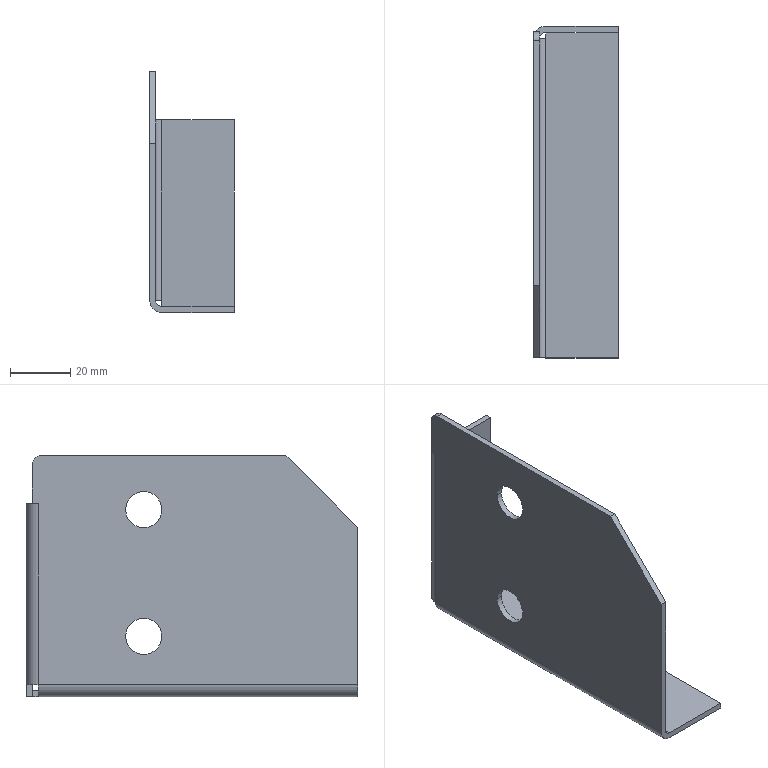Part | NX | features solid 2 | 1 solid | 30 faces | box 28 x 110 x 80 mm | volume 24962 mm3 | plane 21 | cylinder 9 | commonest cylinder face diameters 12 x4 4 x2 8 x2 6 x1
STEP:
#1=CARTESIAN_POINT('',(1138.,-1578.,1213.));
#2=VERTEX_POINT('',#1);
#3=CARTESIAN_POINT('',(1114.,-1578.,1213.));
#4=VERTEX_POINT('',#3);
#5=CARTESIAN_POINT('',(1111.722,-1578.,1213.));
#6=DIRECTION('',(-1.,0.,0.));
#7=VECTOR('',#6,1000.);
#8=LINE('',#5,#7);
#9=EDGE_CURVE('',#2,#4,#8,.T.);
#10=ORIENTED_EDGE('',*,*,#9,.T.);
#11=CARTESIAN_POINT('',(1114.,-1472.,1213.));
#12=VERTEX_POINT('',#11);
#13=CARTESIAN_POINT('',(1114.,-1578.,1213.));
#14=DIRECTION('',(0.,1.,0.));
#15=VECTOR('',#14,1000.);
#16=LINE('',#13,#15);
#17=EDGE_CURVE('',#4,#12,#16,.T.);
#18=ORIENTED_EDGE('',*,*,#17,.T.);
#19=CARTESIAN_POINT('',(1114.,-1470.2,1213.));
#20=VERTEX_POINT('',#19);
#21=CARTESIAN_POINT('',(1114.,-1578.,1213.));
#22=DIRECTION('',(0.,1.,0.));
#23=VECTOR('',#22,1000.);
#24=LINE('',#21,#23);
#25=EDGE_CURVE('',#12,#20,#24,.T.);
#26=ORIENTED_EDGE('',*,*,#25,.T.);
#27=CARTESIAN_POINT('',(1138.,-1470.2,1213.));
#28=VERTEX_POINT('',#27);
#29=CARTESIAN_POINT('',(1111.722,-1470.2,1213.));
#30=DIRECTION('',(1.,0.,0.));
#31=VECTOR('',#30,1000.);
#32=LINE('',#29,#31);
#33=EDGE_CURVE('',#20,#28,#32,.T.);
#34=ORIENTED_EDGE('',*,*,#33,.T.);
#35=CARTESIAN_POINT('',(1138.,-1472.,1213.));
#36=DIRECTION('',(0.,-1.,0.));
#37=VECTOR('',#36,1000.);
#38=LINE('',#35,#37);
#39=EDGE_CURVE('',#28,#2,#38,.T.);
#40=ORIENTED_EDGE('',*,*,#39,.T.);
#41=EDGE_LOOP('',(#10,#18,#26,#34,#40));
#42=FACE_BOUND('',#41,.T.);
#43=CARTESIAN_POINT('',(1110.,-1682.,1213.));
#44=DIRECTION('',(0.,0.,-1.));
#45=DIRECTION('',(0.,-1.,0.));
#46=AXIS2_PLACEMENT_3D('',#43,#44,#45);
#47=PLANE('',#46);
#48=ADVANCED_FACE('',(#42),#47,.T.);
#49=CARTESIAN_POINT('',(1114.,-1578.,1215.));
#50=VERTEX_POINT('',#49);
#51=CARTESIAN_POINT('',(1114.,-1472.,1215.));
#52=VERTEX_POINT('',#51);
#53=CARTESIAN_POINT('',(1114.,-1578.,1215.));
#54=DIRECTION('',(0.,1.,0.));
#55=VECTOR('',#54,1000.);
#56=LINE('',#53,#55);
#57=EDGE_CURVE('',#50,#52,#56,.T.);
#58=ORIENTED_EDGE('',*,*,#57,.F.);
#59=CARTESIAN_POINT('',(1138.,-1578.,1215.));
#60=VERTEX_POINT('',#59);
#61=CARTESIAN_POINT('',(1111.722,-1578.,1215.));
#62=DIRECTION('',(-1.,0.,0.));
#63=VECTOR('',#62,1000.);
#64=LINE('',#61,#63);
#65=EDGE_CURVE('',#60,#50,#64,.T.);
#66=ORIENTED_EDGE('',*,*,#65,.F.);
#67=CARTESIAN_POINT('',(1138.,-1470.2,1215.));
#68=VERTEX_POINT('',#67);
#69=CARTESIAN_POINT('',(1138.,-1472.,1215.));
#70=DIRECTION('',(0.,-1.,0.));
#71=VECTOR('',#70,1000.);
#72=LINE('',#69,#71);
#73=EDGE_CURVE('',#68,#60,#72,.T.);
#74=ORIENTED_EDGE('',*,*,#73,.F.);
#75=CARTESIAN_POINT('',(1114.,-1470.2,1215.));
#76=VERTEX_POINT('',#75);
#77=CARTESIAN_POINT('',(1111.722,-1470.2,1215.));
#78=DIRECTION('',(1.,0.,0.));
#79=VECTOR('',#78,1000.);
#80=LINE('',#77,#79);
#81=EDGE_CURVE('',#76,#68,#80,.T.);
#82=ORIENTED_EDGE('',*,*,#81,.F.);
#83=CARTESIAN_POINT('',(1114.,-1578.,1215.));
#84=DIRECTION('',(0.,1.,0.));
#85=VECTOR('',#84,1000.);
#86=LINE('',#83,#85);
#87=EDGE_CURVE('',#52,#76,#86,.T.);
#88=ORIENTED_EDGE('',*,*,#87,.F.);
#89=EDGE_LOOP('',(#58,#66,#74,#82,#88));
#90=FACE_BOUND('',#89,.T.);
#91=CARTESIAN_POINT('',(1110.,-1682.,1215.));
#92=DIRECTION('',(0.,0.,-1.));
#93=DIRECTION('',(0.,-1.,0.));
#94=AXIS2_PLACEMENT_3D('',#91,#92,#93);
#95=PLANE('',#94);
#96=ADVANCED_FACE('',(#90),#95,.F.);
#97=ORIENTED_EDGE('',*,*,#33,.F.);
#98=CARTESIAN_POINT('',(1114.,-1470.2,1213.));
#99=DIRECTION('',(0.,0.,1.));
#100=VECTOR('',#99,1000.);
#101=LINE('',#98,#100);
#102=EDGE_CURVE('',#20,#76,#101,.T.);
#103=ORIENTED_EDGE('',*,*,#102,.T.);
#104=ORIENTED_EDGE('',*,*,#81,.T.);
#105=CARTESIAN_POINT('',(1138.,-1470.2,1213.));
#106=DIRECTION('',(0.,0.,1.));
#107=VECTOR('',#106,1000.);
#108=LINE('',#105,#107);
#109=EDGE_CURVE('',#28,#68,#108,.T.);
#110=ORIENTED_EDGE('',*,*,#109,.F.);
#111=EDGE_LOOP('',(#97,#103,#104,#110));
#112=FACE_BOUND('',#111,.T.);
#113=CARTESIAN_POINT('',(1111.722,-1470.2,1213.));
#114=DIRECTION('',(0.,-1.,0.));
#115=DIRECTION('',(-1.,0.,0.));
#116=AXIS2_PLACEMENT_3D('',#113,#114,#115);
#117=PLANE('',#116);
#118=ADVANCED_FACE('',(#112),#117,.F.);
#119=ORIENTED_EDGE('',*,*,#73,.T.);
#120=CARTESIAN_POINT('',(1138.,-1578.,1213.));
#121=DIRECTION('',(0.,0.,1.));
#122=VECTOR('',#121,1000.);
#123=LINE('',#120,#122);
#124=EDGE_CURVE('',#2,#60,#123,.T.);
#125=ORIENTED_EDGE('',*,*,#124,.F.);
#126=ORIENTED_EDGE('',*,*,#39,.F.);
#127=ORIENTED_EDGE('',*,*,#109,.T.);
#128=EDGE_LOOP('',(#119,#125,#126,#127));
#129=FACE_BOUND('',#128,.T.);
#130=CARTESIAN_POINT('',(1138.,-1472.,1213.));
#131=DIRECTION('',(-1.,0.,0.));
#132=DIRECTION('',(0.,0.,1.));
#133=AXIS2_PLACEMENT_3D('',#130,#131,#132);
#134=PLANE('',#133);
#135=ADVANCED_FACE('',(#129),#134,.F.);
#136=ORIENTED_EDGE('',*,*,#25,.F.);
#137=CARTESIAN_POINT('',(1114.,-1472.,1213.));
#138=DIRECTION('',(0.,0.,1.));
#139=VECTOR('',#138,1000.);
#140=LINE('',#137,#139);
#141=EDGE_CURVE('',#12,#52,#140,.T.);
#142=ORIENTED_EDGE('',*,*,#141,.T.);
#143=ORIENTED_EDGE('',*,*,#87,.T.);
#144=ORIENTED_EDGE('',*,*,#102,.F.);
#145=EDGE_LOOP('',(#136,#142,#143,#144));
#146=FACE_BOUND('',#145,.T.);
#147=CARTESIAN_POINT('',(1114.,-1682.,0.));
#148=DIRECTION('',(-1.,0.,0.));
#149=DIRECTION('',(0.,1.,0.));
#150=AXIS2_PLACEMENT_3D('',#147,#148,#149);
#151=PLANE('',#150);
#152=ADVANCED_FACE('',(#146),#151,.T.);
#153=CARTESIAN_POINT('',(1110.,-1513.,1275.));
#154=VERTEX_POINT('',#153);
#155=CARTESIAN_POINT('',(1110.,-1501.,1275.));
#156=VERTEX_POINT('',#155);
#157=CARTESIAN_POINT('',(1110.,-1507.,1275.));
#158=DIRECTION('',(1.,0.,0.));
#159=DIRECTION('',(0.,-1.,0.));
#160=AXIS2_PLACEMENT_3D('',#157,#158,#159);
#161=CIRCLE('',#160,6.);
#162=EDGE_CURVE('',#154,#156,#161,.T.);
#163=ORIENTED_EDGE('',*,*,#162,.T.);
#164=CARTESIAN_POINT('',(1110.,-1507.,1275.));
#165=DIRECTION('',(1.,0.,0.));
#166=DIRECTION('',(0.,-1.,0.));
#167=AXIS2_PLACEMENT_3D('',#164,#165,#166);
#168=CIRCLE('',#167,6.);
#169=EDGE_CURVE('',#156,#154,#168,.T.);
#170=ORIENTED_EDGE('',*,*,#169,.T.);
#171=EDGE_LOOP('',(#163,#170));
#172=FACE_BOUND('',#171,.T.);
#173=CARTESIAN_POINT('',(1110.,-1513.,1233.));
#174=VERTEX_POINT('',#173);
#175=CARTESIAN_POINT('',(1110.,-1501.,1233.));
#176=VERTEX_POINT('',#175);
#177=CARTESIAN_POINT('',(1110.,-1507.,1233.));
#178=DIRECTION('',(1.,0.,0.));
#179=DIRECTION('',(0.,-1.,0.));
#180=AXIS2_PLACEMENT_3D('',#177,#178,#179);
#181=CIRCLE('',#180,6.);
#182=EDGE_CURVE('',#174,#176,#181,.T.);
#183=ORIENTED_EDGE('',*,*,#182,.T.);
#184=CARTESIAN_POINT('',(1110.,-1507.,1233.));
#185=DIRECTION('',(1.,0.,0.));
#186=DIRECTION('',(0.,-1.,0.));
#187=AXIS2_PLACEMENT_3D('',#184,#185,#186);
#188=CIRCLE('',#187,6.);
#189=EDGE_CURVE('',#176,#174,#188,.T.);
#190=ORIENTED_EDGE('',*,*,#189,.T.);
#191=EDGE_LOOP('',(#183,#190));
#192=FACE_BOUND('',#191,.T.);
#193=CARTESIAN_POINT('',(1110.,-1472.,1277.));
#194=VERTEX_POINT('',#193);
#195=CARTESIAN_POINT('',(1110.,-1472.,1217.));
#196=VERTEX_POINT('',#195);
#197=CARTESIAN_POINT('',(1110.,-1472.,1277.));
#198=DIRECTION('',(0.,0.,-1.));
#199=VECTOR('',#198,1000.);
#200=LINE('',#197,#199);
#201=EDGE_CURVE('',#194,#196,#200,.T.);
#202=ORIENTED_EDGE('',*,*,#201,.T.);
#203=CARTESIAN_POINT('',(1110.,-1578.,1217.));
#204=VERTEX_POINT('',#203);
#205=CARTESIAN_POINT('',(1110.,-1472.,1217.));
#206=DIRECTION('',(0.,-1.,0.));
#207=VECTOR('',#206,1000.);
#208=LINE('',#205,#207);
#209=EDGE_CURVE('',#196,#204,#208,.T.);
#210=ORIENTED_EDGE('',*,*,#209,.T.);
#211=CARTESIAN_POINT('',(1110.,-1578.,1269.17));
#212=VERTEX_POINT('',#211);
#213=CARTESIAN_POINT('',(1110.,-1578.,1269.17));
#214=DIRECTION('',(0.,0.,-1.));
#215=VECTOR('',#214,1000.);
#216=LINE('',#213,#215);
#217=EDGE_CURVE('',#212,#204,#216,.T.);
#218=ORIENTED_EDGE('',*,*,#217,.F.);
#219=CARTESIAN_POINT('',(1110.,-1554.17,1293.));
#220=VERTEX_POINT('',#219);
#221=CARTESIAN_POINT('',(1110.,-1554.17,1293.));
#222=DIRECTION('',(0.,-0.7071,-0.7071));
#223=VECTOR('',#222,1000.);
#224=LINE('',#221,#223);
#225=EDGE_CURVE('',#220,#212,#224,.T.);
#226=ORIENTED_EDGE('',*,*,#225,.F.);
#227=CARTESIAN_POINT('',(1110.,-1473.,1293.));
#228=VERTEX_POINT('',#227);
#229=CARTESIAN_POINT('',(1110.,-1470.,1293.));
#230=DIRECTION('',(0.,-1.,0.));
#231=VECTOR('',#230,1000.);
#232=LINE('',#229,#231);
#233=EDGE_CURVE('',#228,#220,#232,.T.);
#234=ORIENTED_EDGE('',*,*,#233,.F.);
#235=CARTESIAN_POINT('',(1110.,-1470.,1290.));
#236=VERTEX_POINT('',#235);
#237=CARTESIAN_POINT('',(1110.,-1473.,1290.));
#238=DIRECTION('',(-1.,0.,0.));
#239=DIRECTION('',(0.,0.,1.));
#240=AXIS2_PLACEMENT_3D('',#237,#238,#239);
#241=CIRCLE('',#240,3.);
#242=EDGE_CURVE('',#228,#236,#241,.T.);
#243=ORIENTED_EDGE('',*,*,#242,.T.);
#244=CARTESIAN_POINT('',(1110.,-1470.,1277.1));
#245=VERTEX_POINT('',#244);
#246=CARTESIAN_POINT('',(1110.,-1470.,1213.));
#247=DIRECTION('',(0.,0.,1.));
#248=VECTOR('',#247,1000.);
#249=LINE('',#246,#248);
#250=EDGE_CURVE('',#245,#236,#249,.T.);
#251=ORIENTED_EDGE('',*,*,#250,.F.);
#252=CARTESIAN_POINT('',(1110.,-1472.1,1277.1));
#253=VERTEX_POINT('',#252);
#254=CARTESIAN_POINT('',(1110.,-1470.,1277.1));
#255=DIRECTION('',(0.,1.,0.));
#256=VECTOR('',#255,1000.);
#257=LINE('',#254,#256);
#258=EDGE_CURVE('',#253,#245,#257,.T.);
#259=ORIENTED_EDGE('',*,*,#258,.F.);
#260=CARTESIAN_POINT('',(1110.,-1472.1,1277.));
#261=VERTEX_POINT('',#260);
#262=CARTESIAN_POINT('',(1110.,-1472.1,1277.1));
#263=DIRECTION('',(0.,0.,1.));
#264=VECTOR('',#263,1000.);
#265=LINE('',#262,#264);
#266=EDGE_CURVE('',#261,#253,#265,.T.);
#267=ORIENTED_EDGE('',*,*,#266,.F.);
#268=CARTESIAN_POINT('',(1110.,-1470.,1277.));
#269=DIRECTION('',(0.,-1.,0.));
#270=VECTOR('',#269,1000.);
#271=LINE('',#268,#270);
#272=EDGE_CURVE('',#194,#261,#271,.T.);
#273=ORIENTED_EDGE('',*,*,#272,.F.);
#274=EDGE_LOOP('',(#202,#210,#218,#226,#234,#243,#251,#259,#267,#273));
#275=FACE_BOUND('',#274,.T.);
#276=CARTESIAN_POINT('',(1110.,-1578.,1269.17));
#277=DIRECTION('',(1.,0.,0.));
#278=DIRECTION('',(0.,0.,1.));
#279=AXIS2_PLACEMENT_3D('',#276,#277,#278);
#280=PLANE('',#279);
#281=ADVANCED_FACE('',(#172,#192,#275),#280,.F.);
#282=CARTESIAN_POINT('',(1112.,-1513.,1275.));
#283=VERTEX_POINT('',#282);
#284=CARTESIAN_POINT('',(1112.,-1501.,1275.));
#285=VERTEX_POINT('',#284);
#286=CARTESIAN_POINT('',(1112.,-1507.,1275.));
#287=DIRECTION('',(1.,0.,0.));
#288=DIRECTION('',(0.,0.,1.));
#289=AXIS2_PLACEMENT_3D('',#286,#287,#288);
#290=CIRCLE('',#289,6.);
#291=EDGE_CURVE('',#283,#285,#290,.T.);
#292=ORIENTED_EDGE('',*,*,#291,.F.);
#293=CARTESIAN_POINT('',(1112.,-1507.,1275.));
#294=DIRECTION('',(1.,0.,0.));
#295=DIRECTION('',(0.,0.,1.));
#296=AXIS2_PLACEMENT_3D('',#293,#294,#295);
#297=CIRCLE('',#296,6.);
#298=EDGE_CURVE('',#285,#283,#297,.T.);
#299=ORIENTED_EDGE('',*,*,#298,.F.);
#300=EDGE_LOOP('',(#292,#299));
#301=FACE_BOUND('',#300,.T.);
#302=CARTESIAN_POINT('',(1112.,-1513.,1233.));
#303=VERTEX_POINT('',#302);
#304=CARTESIAN_POINT('',(1112.,-1501.,1233.));
#305=VERTEX_POINT('',#304);
#306=CARTESIAN_POINT('',(1112.,-1507.,1233.));
#307=DIRECTION('',(1.,0.,0.));
#308=DIRECTION('',(0.,0.,1.));
#309=AXIS2_PLACEMENT_3D('',#306,#307,#308);
#310=CIRCLE('',#309,6.);
#311=EDGE_CURVE('',#303,#305,#310,.T.);
#312=ORIENTED_EDGE('',*,*,#311,.F.);
#313=CARTESIAN_POINT('',(1112.,-1507.,1233.));
#314=DIRECTION('',(1.,0.,0.));
#315=DIRECTION('',(0.,0.,1.));
#316=AXIS2_PLACEMENT_3D('',#313,#314,#315);
#317=CIRCLE('',#316,6.);
#318=EDGE_CURVE('',#305,#303,#317,.T.);
#319=ORIENTED_EDGE('',*,*,#318,.F.);
#320=EDGE_LOOP('',(#312,#319));
#321=FACE_BOUND('',#320,.T.);
#322=CARTESIAN_POINT('',(1112.,-1472.,1217.));
#323=VERTEX_POINT('',#322);
#324=CARTESIAN_POINT('',(1112.,-1578.,1217.));
#325=VERTEX_POINT('',#324);
#326=CARTESIAN_POINT('',(1112.,-1472.,1217.));
#327=DIRECTION('',(0.,-1.,0.));
#328=VECTOR('',#327,1000.);
#329=LINE('',#326,#328);
#330=EDGE_CURVE('',#323,#325,#329,.T.);
#331=ORIENTED_EDGE('',*,*,#330,.F.);
#332=CARTESIAN_POINT('',(1112.,-1472.,1277.));
#333=VERTEX_POINT('',#332);
#334=CARTESIAN_POINT('',(1112.,-1472.,1277.));
#335=DIRECTION('',(0.,0.,-1.));
#336=VECTOR('',#335,1000.);
#337=LINE('',#334,#336);
#338=EDGE_CURVE('',#333,#323,#337,.T.);
#339=ORIENTED_EDGE('',*,*,#338,.F.);
#340=CARTESIAN_POINT('',(1112.,-1472.1,1277.));
#341=VERTEX_POINT('',#340);
#342=CARTESIAN_POINT('',(1112.,-1472.1,1277.));
#343=DIRECTION('',(0.,-1.,0.));
#344=VECTOR('',#343,1000.);
#345=LINE('',#342,#344);
#346=EDGE_CURVE('',#333,#341,#345,.T.);
#347=ORIENTED_EDGE('',*,*,#346,.T.);
#348=CARTESIAN_POINT('',(1112.,-1472.1,1277.1));
#349=VERTEX_POINT('',#348);
#350=CARTESIAN_POINT('',(1112.,-1472.1,1277.));
#351=DIRECTION('',(0.,0.,1.));
#352=VECTOR('',#351,1000.);
#353=LINE('',#350,#352);
#354=EDGE_CURVE('',#341,#349,#353,.T.);
#355=ORIENTED_EDGE('',*,*,#354,.T.);
#356=CARTESIAN_POINT('',(1112.,-1470.,1277.1));
#357=VERTEX_POINT('',#356);
#358=CARTESIAN_POINT('',(1112.,-1472.1,1277.1));
#359=DIRECTION('',(0.,1.,0.));
#360=VECTOR('',#359,1000.);
#361=LINE('',#358,#360);
#362=EDGE_CURVE('',#349,#357,#361,.T.);
#363=ORIENTED_EDGE('',*,*,#362,.T.);
#364=CARTESIAN_POINT('',(1112.,-1470.,1290.));
#365=VERTEX_POINT('',#364);
#366=CARTESIAN_POINT('',(1112.,-1470.,1213.));
#367=DIRECTION('',(0.,0.,1.));
#368=VECTOR('',#367,1000.);
#369=LINE('',#366,#368);
#370=EDGE_CURVE('',#357,#365,#369,.T.);
#371=ORIENTED_EDGE('',*,*,#370,.T.);
#372=CARTESIAN_POINT('',(1112.,-1473.,1293.));
#373=VERTEX_POINT('',#372);
#374=CARTESIAN_POINT('',(1112.,-1473.,1290.));
#375=DIRECTION('',(1.,0.,0.));
#376=DIRECTION('',(0.,0.,1.));
#377=AXIS2_PLACEMENT_3D('',#374,#375,#376);
#378=CIRCLE('',#377,3.);
#379=EDGE_CURVE('',#365,#373,#378,.T.);
#380=ORIENTED_EDGE('',*,*,#379,.T.);
#381=CARTESIAN_POINT('',(1112.,-1554.17,1293.));
#382=VERTEX_POINT('',#381);
#383=CARTESIAN_POINT('',(1112.,-1470.,1293.));
#384=DIRECTION('',(0.,-1.,0.));
#385=VECTOR('',#384,1000.);
#386=LINE('',#383,#385);
#387=EDGE_CURVE('',#373,#382,#386,.T.);
#388=ORIENTED_EDGE('',*,*,#387,.T.);
#389=CARTESIAN_POINT('',(1112.,-1578.,1269.17));
#390=VERTEX_POINT('',#389);
#391=CARTESIAN_POINT('',(1112.,-1554.17,1293.));
#392=DIRECTION('',(0.,-0.7071,-0.7071));
#393=VECTOR('',#392,1000.);
#394=LINE('',#391,#393);
#395=EDGE_CURVE('',#382,#390,#394,.T.);
#396=ORIENTED_EDGE('',*,*,#395,.T.);
#397=CARTESIAN_POINT('',(1112.,-1578.,1269.17));
#398=DIRECTION('',(0.,0.,-1.));
#399=VECTOR('',#398,1000.);
#400=LINE('',#397,#399);
#401=EDGE_CURVE('',#390,#325,#400,.T.);
#402=ORIENTED_EDGE('',*,*,#401,.T.);
#403=EDGE_LOOP('',(#331,#339,#347,#355,#363,#371,#380,#388,#396,#402));
#404=FACE_BOUND('',#403,.T.);
#405=CARTESIAN_POINT('',(1112.,-1578.,1269.17));
#406=DIRECTION('',(1.,0.,0.));
#407=DIRECTION('',(0.,0.,1.));
#408=AXIS2_PLACEMENT_3D('',#405,#406,#407);
#409=PLANE('',#408);
#410=ADVANCED_FACE('',(#301,#321,#404),#409,.T.);
#411=ORIENTED_EDGE('',*,*,#354,.F.);
#412=CARTESIAN_POINT('',(1110.,-1472.1,1277.));
#413=DIRECTION('',(-1.,0.,0.));
#414=VECTOR('',#413,1000.);
#415=LINE('',#412,#414);
#416=EDGE_CURVE('',#341,#261,#415,.T.);
#417=ORIENTED_EDGE('',*,*,#416,.T.);
#418=ORIENTED_EDGE('',*,*,#266,.T.);
#419=CARTESIAN_POINT('',(1110.,-1472.1,1277.1));
#420=DIRECTION('',(-1.,0.,0.));
#421=VECTOR('',#420,1000.);
#422=LINE('',#419,#421);
#423=EDGE_CURVE('',#349,#253,#422,.T.);
#424=ORIENTED_EDGE('',*,*,#423,.F.);
#425=EDGE_LOOP('',(#411,#417,#418,#424));
#426=FACE_BOUND('',#425,.T.);
#427=CARTESIAN_POINT('',(1110.,-1472.1,1277.1));
#428=DIRECTION('',(0.,-1.,0.));
#429=DIRECTION('',(-1.,0.,0.));
#430=AXIS2_PLACEMENT_3D('',#427,#428,#429);
#431=PLANE('',#430);
#432=ADVANCED_FACE('',(#426),#431,.F.);
#433=ORIENTED_EDGE('',*,*,#423,.T.);
#434=ORIENTED_EDGE('',*,*,#258,.T.);
#435=CARTESIAN_POINT('',(1110.,-1470.,1277.1));
#436=DIRECTION('',(-1.,0.,0.));
#437=VECTOR('',#436,1000.);
#438=LINE('',#435,#437);
#439=EDGE_CURVE('',#357,#245,#438,.T.);
#440=ORIENTED_EDGE('',*,*,#439,.F.);
#441=ORIENTED_EDGE('',*,*,#362,.F.);
#442=EDGE_LOOP('',(#433,#434,#440,#441));
#443=FACE_BOUND('',#442,.T.);
#444=CARTESIAN_POINT('',(1110.,-1470.,1277.1));
#445=DIRECTION('',(0.,0.,1.));
#446=DIRECTION('',(1.,0.,0.));
#447=AXIS2_PLACEMENT_3D('',#444,#445,#446);
#448=PLANE('',#447);
#449=ADVANCED_FACE('',(#443),#448,.F.);
#450=ORIENTED_EDGE('',*,*,#250,.T.);
#451=CARTESIAN_POINT('',(1112.,-1470.,1290.));
#452=DIRECTION('',(1.,0.,0.));
#453=VECTOR('',#452,1000.);
#454=LINE('',#451,#453);
#455=EDGE_CURVE('',#236,#365,#454,.T.);
#456=ORIENTED_EDGE('',*,*,#455,.T.);
#457=ORIENTED_EDGE('',*,*,#370,.F.);
#458=ORIENTED_EDGE('',*,*,#439,.T.);
#459=EDGE_LOOP('',(#450,#456,#457,#458));
#460=FACE_BOUND('',#459,.T.);
#461=CARTESIAN_POINT('',(1112.,-1470.,1213.));
#462=DIRECTION('',(0.,-1.,0.));
#463=DIRECTION('',(-1.,0.,0.));
#464=AXIS2_PLACEMENT_3D('',#461,#462,#463);
#465=PLANE('',#464);
#466=ADVANCED_FACE('',(#460),#465,.F.);
#467=ORIENTED_EDGE('',*,*,#379,.F.);
#468=ORIENTED_EDGE('',*,*,#455,.F.);
#469=ORIENTED_EDGE('',*,*,#242,.F.);
#470=CARTESIAN_POINT('',(1112.,-1473.,1293.));
#471=DIRECTION('',(-1.,0.,0.));
#472=VECTOR('',#471,1000.);
#473=LINE('',#470,#472);
#474=EDGE_CURVE('',#373,#228,#473,.T.);
#475=ORIENTED_EDGE('',*,*,#474,.F.);
#476=EDGE_LOOP('',(#467,#468,#469,#475));
#477=FACE_BOUND('',#476,.T.);
#478=CARTESIAN_POINT('',(1112.,-1473.,1290.));
#479=DIRECTION('',(-1.,0.,0.));
#480=DIRECTION('',(0.,0.,-1.));
#481=AXIS2_PLACEMENT_3D('',#478,#479,#480);
#482=CYLINDRICAL_SURFACE('',#481,3.);
#483=ADVANCED_FACE('',(#477),#482,.T.);
#484=ORIENTED_EDGE('',*,*,#387,.F.);
#485=ORIENTED_EDGE('',*,*,#474,.T.);
#486=ORIENTED_EDGE('',*,*,#233,.T.);
#487=CARTESIAN_POINT('',(1112.,-1554.17,1293.));
#488=DIRECTION('',(-1.,0.,0.));
#489=VECTOR('',#488,1000.);
#490=LINE('',#487,#489);
#491=EDGE_CURVE('',#382,#220,#490,.T.);
#492=ORIENTED_EDGE('',*,*,#491,.F.);
#493=EDGE_LOOP('',(#484,#485,#486,#492));
#494=FACE_BOUND('',#493,.T.);
#495=CARTESIAN_POINT('',(1112.,-1470.,1293.));
#496=DIRECTION('',(0.,0.,-1.));
#497=DIRECTION('',(0.,-1.,0.));
#498=AXIS2_PLACEMENT_3D('',#495,#496,#497);
#499=PLANE('',#498);
#500=ADVANCED_FACE('',(#494),#499,.F.);
#501=ORIENTED_EDGE('',*,*,#225,.T.);
#502=CARTESIAN_POINT('',(1112.,-1578.,1269.17));
#503=DIRECTION('',(-1.,0.,0.));
#504=VECTOR('',#503,1000.);
#505=LINE('',#502,#504);
#506=EDGE_CURVE('',#390,#212,#505,.T.);
#507=ORIENTED_EDGE('',*,*,#506,.F.);
#508=ORIENTED_EDGE('',*,*,#395,.F.);
#509=ORIENTED_EDGE('',*,*,#491,.T.);
#510=EDGE_LOOP('',(#501,#507,#508,#509));
#511=FACE_BOUND('',#510,.T.);
#512=CARTESIAN_POINT('',(1112.,-1554.17,1293.));
#513=DIRECTION('',(0.,0.7071,-0.7071));
#514=DIRECTION('',(-1.,0.,0.));
#515=AXIS2_PLACEMENT_3D('',#512,#513,#514);
#516=PLANE('',#515);
#517=ADVANCED_FACE('',(#511),#516,.F.);
#518=CARTESIAN_POINT('',(1110.,-1501.,1233.));
#519=DIRECTION('',(1.,0.,0.));
#520=VECTOR('',#519,1000.);
#521=LINE('',#518,#520);
#522=EDGE_CURVE('',#305,#176,#521,.F.);
#523=ORIENTED_EDGE('',*,*,#522,.T.);
#524=ORIENTED_EDGE('',*,*,#182,.F.);
#525=CARTESIAN_POINT('',(1110.,-1513.,1233.));
#526=DIRECTION('',(1.,0.,0.));
#527=VECTOR('',#526,1000.);
#528=LINE('',#525,#527);
#529=EDGE_CURVE('',#174,#303,#528,.T.);
#530=ORIENTED_EDGE('',*,*,#529,.T.);
#531=ORIENTED_EDGE('',*,*,#311,.T.);
#532=EDGE_LOOP('',(#523,#524,#530,#531));
#533=FACE_BOUND('',#532,.T.);
#534=CARTESIAN_POINT('',(1110.,-1507.,1233.));
#535=DIRECTION('',(1.,0.,0.));
#536=DIRECTION('',(0.,-1.,0.));
#537=AXIS2_PLACEMENT_3D('',#534,#535,#536);
#538=CYLINDRICAL_SURFACE('',#537,6.);
#539=ADVANCED_FACE('',(#533),#538,.F.);
#540=CARTESIAN_POINT('',(1110.,-1501.,1275.));
#541=DIRECTION('',(1.,0.,0.));
#542=VECTOR('',#541,1000.);
#543=LINE('',#540,#542);
#544=EDGE_CURVE('',#285,#156,#543,.F.);
#545=ORIENTED_EDGE('',*,*,#544,.T.);
#546=ORIENTED_EDGE('',*,*,#162,.F.);
#547=CARTESIAN_POINT('',(1110.,-1513.,1275.));
#548=DIRECTION('',(1.,0.,0.));
#549=VECTOR('',#548,1000.);
#550=LINE('',#547,#549);
#551=EDGE_CURVE('',#154,#283,#550,.T.);
#552=ORIENTED_EDGE('',*,*,#551,.T.);
#553=ORIENTED_EDGE('',*,*,#291,.T.);
#554=EDGE_LOOP('',(#545,#546,#552,#553));
#555=FACE_BOUND('',#554,.T.);
#556=CARTESIAN_POINT('',(1110.,-1507.,1275.));
#557=DIRECTION('',(1.,0.,0.));
#558=DIRECTION('',(0.,-1.,0.));
#559=AXIS2_PLACEMENT_3D('',#556,#557,#558);
#560=CYLINDRICAL_SURFACE('',#559,6.);
#561=ADVANCED_FACE('',(#555),#560,.F.);
#562=ORIENTED_EDGE('',*,*,#141,.F.);
#563=CARTESIAN_POINT('',(1114.,-1472.,1217.));
#564=DIRECTION('',(0.,-1.,0.));
#565=DIRECTION('',(1.,0.,0.));
#566=AXIS2_PLACEMENT_3D('',#563,#564,#565);
#567=CIRCLE('',#566,4.);
#568=EDGE_CURVE('',#196,#12,#567,.T.);
#569=ORIENTED_EDGE('',*,*,#568,.F.);
#570=CARTESIAN_POINT('',(1110.,-1472.,1217.));
#571=DIRECTION('',(-1.,0.,0.));
#572=VECTOR('',#571,1000.);
#573=LINE('',#570,#572);
#574=EDGE_CURVE('',#323,#196,#573,.T.);
#575=ORIENTED_EDGE('',*,*,#574,.F.);
#576=CARTESIAN_POINT('',(1114.,-1472.,1217.));
#577=DIRECTION('',(0.,-1.,0.));
#578=DIRECTION('',(0.,0.,-1.));
#579=AXIS2_PLACEMENT_3D('',#576,#577,#578);
#580=CIRCLE('',#579,2.);
#581=EDGE_CURVE('',#323,#52,#580,.T.);
#582=ORIENTED_EDGE('',*,*,#581,.T.);
#583=EDGE_LOOP('',(#562,#569,#575,#582));
#584=FACE_BOUND('',#583,.T.);
#585=CARTESIAN_POINT('',(1111.722,-1472.,1213.));
#586=DIRECTION('',(0.,-1.,0.));
#587=DIRECTION('',(-1.,0.,0.));
#588=AXIS2_PLACEMENT_3D('',#585,#586,#587);
#589=PLANE('',#588);
#590=ADVANCED_FACE('',(#584),#589,.F.);
#591=ORIENTED_EDGE('',*,*,#330,.T.);
#592=CARTESIAN_POINT('',(1114.,-1578.,1217.));
#593=DIRECTION('',(0.,-1.,0.));
#594=DIRECTION('',(0.,0.,-1.));
#595=AXIS2_PLACEMENT_3D('',#592,#593,#594);
#596=CIRCLE('',#595,2.);
#597=EDGE_CURVE('',#325,#50,#596,.T.);
#598=ORIENTED_EDGE('',*,*,#597,.T.);
#599=ORIENTED_EDGE('',*,*,#57,.T.);
#600=ORIENTED_EDGE('',*,*,#581,.F.);
#601=EDGE_LOOP('',(#591,#598,#599,#600));
#602=FACE_BOUND('',#601,.T.);
#603=CARTESIAN_POINT('',(1114.,-1472.,1217.));
#604=DIRECTION('',(0.,-1.,0.));
#605=DIRECTION('',(1.,0.,0.));
#606=AXIS2_PLACEMENT_3D('',#603,#604,#605);
#607=CYLINDRICAL_SURFACE('',#606,2.);
#608=ADVANCED_FACE('',(#602),#607,.F.);
#609=CARTESIAN_POINT('',(1114.,-1578.,1217.));
#610=DIRECTION('',(0.,-1.,0.));
#611=DIRECTION('',(1.,0.,0.));
#612=AXIS2_PLACEMENT_3D('',#609,#610,#611);
#613=CIRCLE('',#612,4.);
#614=EDGE_CURVE('',#204,#4,#613,.T.);
#615=ORIENTED_EDGE('',*,*,#614,.T.);
#616=ORIENTED_EDGE('',*,*,#9,.F.);
#617=ORIENTED_EDGE('',*,*,#124,.T.);
#618=ORIENTED_EDGE('',*,*,#65,.T.);
#619=ORIENTED_EDGE('',*,*,#597,.F.);
#620=ORIENTED_EDGE('',*,*,#401,.F.);
#621=ORIENTED_EDGE('',*,*,#506,.T.);
#622=ORIENTED_EDGE('',*,*,#217,.T.);
#623=EDGE_LOOP('',(#615,#616,#617,#618,#619,#620,#621,#622));
#624=FACE_BOUND('',#623,.T.);
#625=CARTESIAN_POINT('',(1112.,-1578.,1269.17));
#626=DIRECTION('',(0.,1.,0.));
#627=DIRECTION('',(0.,0.,-1.));
#628=AXIS2_PLACEMENT_3D('',#625,#626,#627);
#629=PLANE('',#628);
#630=ADVANCED_FACE('',(#624),#629,.F.);
#631=ORIENTED_EDGE('',*,*,#209,.F.);
#632=ORIENTED_EDGE('',*,*,#568,.T.);
#633=ORIENTED_EDGE('',*,*,#17,.F.);
#634=ORIENTED_EDGE('',*,*,#614,.F.);
#635=EDGE_LOOP('',(#631,#632,#633,#634));
#636=FACE_BOUND('',#635,.T.);
#637=CARTESIAN_POINT('',(1114.,-1472.,1217.));
#638=DIRECTION('',(0.,-1.,0.));
#639=DIRECTION('',(1.,0.,0.));
#640=AXIS2_PLACEMENT_3D('',#637,#638,#639);
#641=CYLINDRICAL_SURFACE('',#640,4.);
#642=ADVANCED_FACE('',(#636),#641,.T.);
#643=CARTESIAN_POINT('',(1114.,-1470.,1217.));
#644=VERTEX_POINT('',#643);
#645=CARTESIAN_POINT('',(1114.,-1472.,1217.));
#646=DIRECTION('',(0.,0.,1.));
#647=DIRECTION('',(0.,1.,0.));
#648=AXIS2_PLACEMENT_3D('',#645,#646,#647);
#649=CIRCLE('',#648,2.);
#650=EDGE_CURVE('',#644,#323,#649,.T.);
#651=ORIENTED_EDGE('',*,*,#650,.T.);
#652=ORIENTED_EDGE('',*,*,#574,.T.);
#653=CARTESIAN_POINT('',(1114.,-1468.,1217.));
#654=VERTEX_POINT('',#653);
#655=CARTESIAN_POINT('',(1114.,-1472.,1217.));
#656=DIRECTION('',(0.,0.,1.));
#657=DIRECTION('',(0.,1.,0.));
#658=AXIS2_PLACEMENT_3D('',#655,#656,#657);
#659=CIRCLE('',#658,4.);
#660=EDGE_CURVE('',#654,#196,#659,.T.);
#661=ORIENTED_EDGE('',*,*,#660,.F.);
#662=CARTESIAN_POINT('',(1114.,-1468.,1217.));
#663=DIRECTION('',(0.,1.,0.));
#664=VECTOR('',#663,1000.);
#665=LINE('',#662,#664);
#666=EDGE_CURVE('',#644,#654,#665,.T.);
#667=ORIENTED_EDGE('',*,*,#666,.F.);
#668=EDGE_LOOP('',(#651,#652,#661,#667));
#669=FACE_BOUND('',#668,.T.);
#670=CARTESIAN_POINT('',(1114.,-1472.,1217.));
#671=DIRECTION('',(0.,0.,-1.));
#672=DIRECTION('',(0.,-1.,0.));
#673=AXIS2_PLACEMENT_3D('',#670,#671,#672);
#674=PLANE('',#673);
#675=ADVANCED_FACE('',(#669),#674,.T.);
#676=ORIENTED_EDGE('',*,*,#650,.F.);
#677=CARTESIAN_POINT('',(1114.,-1470.,1277.));
#678=VERTEX_POINT('',#677);
#679=CARTESIAN_POINT('',(1114.,-1470.,1213.));
#680=DIRECTION('',(0.,0.,1.));
#681=VECTOR('',#680,1000.);
#682=LINE('',#679,#681);
#683=EDGE_CURVE('',#644,#678,#682,.T.);
#684=ORIENTED_EDGE('',*,*,#683,.T.);
#685=CARTESIAN_POINT('',(1114.,-1472.,1277.));
#686=DIRECTION('',(0.,0.,1.));
#687=DIRECTION('',(0.,1.,0.));
#688=AXIS2_PLACEMENT_3D('',#685,#686,#687);
#689=CIRCLE('',#688,2.);
#690=EDGE_CURVE('',#678,#333,#689,.T.);
#691=ORIENTED_EDGE('',*,*,#690,.T.);
#692=ORIENTED_EDGE('',*,*,#338,.T.);
#693=EDGE_LOOP('',(#676,#684,#691,#692));
#694=FACE_BOUND('',#693,.T.);
#695=CARTESIAN_POINT('',(1114.,-1472.,1277.));
#696=DIRECTION('',(0.,0.,-1.));
#697=DIRECTION('',(1.,0.,0.));
#698=AXIS2_PLACEMENT_3D('',#695,#696,#697);
#699=CYLINDRICAL_SURFACE('',#698,2.);
#700=ADVANCED_FACE('',(#694),#699,.F.);
#701=CARTESIAN_POINT('',(1114.,-1468.,1277.));
#702=VERTEX_POINT('',#701);
#703=CARTESIAN_POINT('',(1114.,-1472.,1277.));
#704=DIRECTION('',(0.,0.,1.));
#705=DIRECTION('',(1.,0.,0.));
#706=AXIS2_PLACEMENT_3D('',#703,#704,#705);
#707=CIRCLE('',#706,4.);
#708=EDGE_CURVE('',#702,#194,#707,.T.);
#709=ORIENTED_EDGE('',*,*,#708,.T.);
#710=ORIENTED_EDGE('',*,*,#272,.T.);
#711=ORIENTED_EDGE('',*,*,#416,.F.);
#712=ORIENTED_EDGE('',*,*,#346,.F.);
#713=ORIENTED_EDGE('',*,*,#690,.F.);
#714=CARTESIAN_POINT('',(1138.,-1470.,1277.));
#715=VERTEX_POINT('',#714);
#716=CARTESIAN_POINT('',(1111.722,-1470.,1277.));
#717=DIRECTION('',(1.,0.,0.));
#718=VECTOR('',#717,1000.);
#719=LINE('',#716,#718);
#720=EDGE_CURVE('',#678,#715,#719,.T.);
#721=ORIENTED_EDGE('',*,*,#720,.T.);
#722=CARTESIAN_POINT('',(1138.,-1468.,1277.));
#723=VERTEX_POINT('',#722);
#724=CARTESIAN_POINT('',(1138.,-1468.,1277.));
#725=DIRECTION('',(0.,-1.,0.));
#726=VECTOR('',#725,1000.);
#727=LINE('',#724,#726);
#728=EDGE_CURVE('',#723,#715,#727,.T.);
#729=ORIENTED_EDGE('',*,*,#728,.F.);
#730=CARTESIAN_POINT('',(1111.722,-1468.,1277.));
#731=DIRECTION('',(1.,0.,0.));
#732=VECTOR('',#731,1000.);
#733=LINE('',#730,#732);
#734=EDGE_CURVE('',#702,#723,#733,.T.);
#735=ORIENTED_EDGE('',*,*,#734,.F.);
#736=EDGE_LOOP('',(#709,#710,#711,#712,#713,#721,#729,#735));
#737=FACE_BOUND('',#736,.T.);
#738=CARTESIAN_POINT('',(1110.,-1470.,1277.));
#739=DIRECTION('',(0.,0.,-1.));
#740=DIRECTION('',(0.,-1.,0.));
#741=AXIS2_PLACEMENT_3D('',#738,#739,#740);
#742=PLANE('',#741);
#743=ADVANCED_FACE('',(#737),#742,.F.);
#744=CARTESIAN_POINT('',(1114.,-1468.,1213.));
#745=DIRECTION('',(0.,0.,1.));
#746=VECTOR('',#745,1000.);
#747=LINE('',#744,#746);
#748=EDGE_CURVE('',#654,#702,#747,.T.);
#749=ORIENTED_EDGE('',*,*,#748,.F.);
#750=ORIENTED_EDGE('',*,*,#660,.T.);
#751=ORIENTED_EDGE('',*,*,#201,.F.);
#752=ORIENTED_EDGE('',*,*,#708,.F.);
#753=EDGE_LOOP('',(#749,#750,#751,#752));
#754=FACE_BOUND('',#753,.T.);
#755=CARTESIAN_POINT('',(1114.,-1472.,1277.));
#756=DIRECTION('',(0.,0.,-1.));
#757=DIRECTION('',(1.,0.,0.));
#758=AXIS2_PLACEMENT_3D('',#755,#756,#757);
#759=CYLINDRICAL_SURFACE('',#758,4.);
#760=ADVANCED_FACE('',(#754),#759,.T.);
#761=CARTESIAN_POINT('',(1114.,-1470.,1213.));
#762=VERTEX_POINT('',#761);
#763=CARTESIAN_POINT('',(1114.,-1470.,1213.));
#764=DIRECTION('',(0.,0.,1.));
#765=VECTOR('',#764,1000.);
#766=LINE('',#763,#765);
#767=EDGE_CURVE('',#762,#644,#766,.T.);
#768=ORIENTED_EDGE('',*,*,#767,.T.);
#769=ORIENTED_EDGE('',*,*,#666,.T.);
#770=CARTESIAN_POINT('',(1114.,-1468.,1213.));
#771=VERTEX_POINT('',#770);
#772=CARTESIAN_POINT('',(1114.,-1468.,1213.));
#773=DIRECTION('',(0.,0.,1.));
#774=VECTOR('',#773,1000.);
#775=LINE('',#772,#774);
#776=EDGE_CURVE('',#771,#654,#775,.T.);
#777=ORIENTED_EDGE('',*,*,#776,.F.);
#778=CARTESIAN_POINT('',(1114.,-1468.,1213.));
#779=DIRECTION('',(0.,-1.,0.));
#780=VECTOR('',#779,1000.);
#781=LINE('',#778,#780);
#782=EDGE_CURVE('',#771,#762,#781,.T.);
#783=ORIENTED_EDGE('',*,*,#782,.T.);
#784=EDGE_LOOP('',(#768,#769,#777,#783));
#785=FACE_BOUND('',#784,.T.);
#786=CARTESIAN_POINT('',(1114.,-1468.,1213.));
#787=DIRECTION('',(1.,0.,0.));
#788=DIRECTION('',(0.,0.,1.));
#789=AXIS2_PLACEMENT_3D('',#786,#787,#788);
#790=PLANE('',#789);
#791=ADVANCED_FACE('',(#785),#790,.F.);
#792=CARTESIAN_POINT('',(1138.,-1470.,1213.));
#793=VERTEX_POINT('',#792);
#794=CARTESIAN_POINT('',(1138.,-1470.,1277.));
#795=DIRECTION('',(0.,0.,-1.));
#796=VECTOR('',#795,1000.);
#797=LINE('',#794,#796);
#798=EDGE_CURVE('',#715,#793,#797,.T.);
#799=ORIENTED_EDGE('',*,*,#798,.T.);
#800=CARTESIAN_POINT('',(1138.,-1468.,1213.));
#801=VERTEX_POINT('',#800);
#802=CARTESIAN_POINT('',(1138.,-1468.,1213.));
#803=DIRECTION('',(0.,-1.,0.));
#804=VECTOR('',#803,1000.);
#805=LINE('',#802,#804);
#806=EDGE_CURVE('',#801,#793,#805,.T.);
#807=ORIENTED_EDGE('',*,*,#806,.F.);
#808=CARTESIAN_POINT('',(1138.,-1468.,1277.));
#809=DIRECTION('',(0.,0.,-1.));
#810=VECTOR('',#809,1000.);
#811=LINE('',#808,#810);
#812=EDGE_CURVE('',#723,#801,#811,.T.);
#813=ORIENTED_EDGE('',*,*,#812,.F.);
#814=ORIENTED_EDGE('',*,*,#728,.T.);
#815=EDGE_LOOP('',(#799,#807,#813,#814));
#816=FACE_BOUND('',#815,.T.);
#817=CARTESIAN_POINT('',(1138.,-1468.,1277.));
#818=DIRECTION('',(-1.,0.,0.));
#819=DIRECTION('',(0.,0.,1.));
#820=AXIS2_PLACEMENT_3D('',#817,#818,#819);
#821=PLANE('',#820);
#822=ADVANCED_FACE('',(#816),#821,.F.);
#823=ORIENTED_EDGE('',*,*,#767,.F.);
#824=CARTESIAN_POINT('',(1111.722,-1470.,1213.));
#825=DIRECTION('',(-1.,0.,0.));
#826=VECTOR('',#825,1000.);
#827=LINE('',#824,#826);
#828=EDGE_CURVE('',#793,#762,#827,.T.);
#829=ORIENTED_EDGE('',*,*,#828,.F.);
#830=ORIENTED_EDGE('',*,*,#798,.F.);
#831=ORIENTED_EDGE('',*,*,#720,.F.);
#832=ORIENTED_EDGE('',*,*,#683,.F.);
#833=EDGE_LOOP('',(#823,#829,#830,#831,#832));
#834=FACE_BOUND('',#833,.T.);
#835=CARTESIAN_POINT('',(1111.722,-1470.,1213.));
#836=DIRECTION('',(0.,1.,0.));
#837=DIRECTION('',(0.,0.,-1.));
#838=AXIS2_PLACEMENT_3D('',#835,#836,#837);
#839=PLANE('',#838);
#840=ADVANCED_FACE('',(#834),#839,.F.);
#841=CARTESIAN_POINT('',(1111.722,-1468.,1213.));
#842=DIRECTION('',(-1.,0.,0.));
#843=VECTOR('',#842,1000.);
#844=LINE('',#841,#843);
#845=EDGE_CURVE('',#801,#771,#844,.T.);
#846=ORIENTED_EDGE('',*,*,#845,.T.);
#847=ORIENTED_EDGE('',*,*,#776,.T.);
#848=ORIENTED_EDGE('',*,*,#748,.T.);
#849=ORIENTED_EDGE('',*,*,#734,.T.);
#850=ORIENTED_EDGE('',*,*,#812,.T.);
#851=EDGE_LOOP('',(#846,#847,#848,#849,#850));
#852=FACE_BOUND('',#851,.T.);
#853=CARTESIAN_POINT('',(1111.722,-1468.,1213.));
#854=DIRECTION('',(0.,1.,0.));
#855=DIRECTION('',(0.,0.,-1.));
#856=AXIS2_PLACEMENT_3D('',#853,#854,#855);
#857=PLANE('',#856);
#858=ADVANCED_FACE('',(#852),#857,.T.);
#859=ORIENTED_EDGE('',*,*,#828,.T.);
#860=ORIENTED_EDGE('',*,*,#782,.F.);
#861=ORIENTED_EDGE('',*,*,#845,.F.);
#862=ORIENTED_EDGE('',*,*,#806,.T.);
#863=EDGE_LOOP('',(#859,#860,#861,#862));
#864=FACE_BOUND('',#863,.T.);
#865=CARTESIAN_POINT('',(1112.,-1470.,1213.));
#866=DIRECTION('',(0.,0.,1.));
#867=DIRECTION('',(1.,0.,0.));
#868=AXIS2_PLACEMENT_3D('',#865,#866,#867);
#869=PLANE('',#868);
#870=ADVANCED_FACE('',(#864),#869,.F.);
#871=ORIENTED_EDGE('',*,*,#169,.F.);
#872=ORIENTED_EDGE('',*,*,#544,.F.);
#873=ORIENTED_EDGE('',*,*,#298,.T.);
#874=ORIENTED_EDGE('',*,*,#551,.F.);
#875=EDGE_LOOP('',(#871,#872,#873,#874));
#876=FACE_BOUND('',#875,.T.);
#877=CARTESIAN_POINT('',(1110.,-1507.,1275.));
#878=DIRECTION('',(1.,0.,0.));
#879=DIRECTION('',(0.,-1.,0.));
#880=AXIS2_PLACEMENT_3D('',#877,#878,#879);
#881=CYLINDRICAL_SURFACE('',#880,6.);
#882=ADVANCED_FACE('',(#876),#881,.F.);
#883=ORIENTED_EDGE('',*,*,#189,.F.);
#884=ORIENTED_EDGE('',*,*,#522,.F.);
#885=ORIENTED_EDGE('',*,*,#318,.T.);
#886=ORIENTED_EDGE('',*,*,#529,.F.);
#887=EDGE_LOOP('',(#883,#884,#885,#886));
#888=FACE_BOUND('',#887,.T.);
#889=CARTESIAN_POINT('',(1110.,-1507.,1233.));
#890=DIRECTION('',(1.,0.,0.));
#891=DIRECTION('',(0.,-1.,0.));
#892=AXIS2_PLACEMENT_3D('',#889,#890,#891);
#893=CYLINDRICAL_SURFACE('',#892,6.);
#894=ADVANCED_FACE('',(#888),#893,.F.);
#895=CLOSED_SHELL('',(#48,#96,#118,#135,#152,#281,#410,#432,#449,#466,#483,#500,#517,#539,#561,#590,#608,#630,#642,#675,#700,#743,#760,#791,#822,#840,#858,#870,#882,#894));
#896=MANIFOLD_SOLID_BREP('',#895);
#897=(LENGTH_UNIT()NAMED_UNIT(*)SI_UNIT(.MILLI.,.METRE.));
#898=UNCERTAINTY_MEASURE_WITH_UNIT(LENGTH_MEASURE(0.00001),#897,'','');
#899=(NAMED_UNIT(*)PLANE_ANGLE_UNIT()SI_UNIT($,.RADIAN.));
#900=(NAMED_UNIT(*)SI_UNIT($,.STERADIAN.)SOLID_ANGLE_UNIT());
#901=(GEOMETRIC_REPRESENTATION_CONTEXT(3)GLOBAL_UNCERTAINTY_ASSIGNED_CONTEXT((#898))GLOBAL_UNIT_ASSIGNED_CONTEXT((#897,#899,#900))REPRESENTATION_CONTEXT('',''));
#902=ADVANCED_BREP_SHAPE_REPRESENTATION('',(#896),#901);